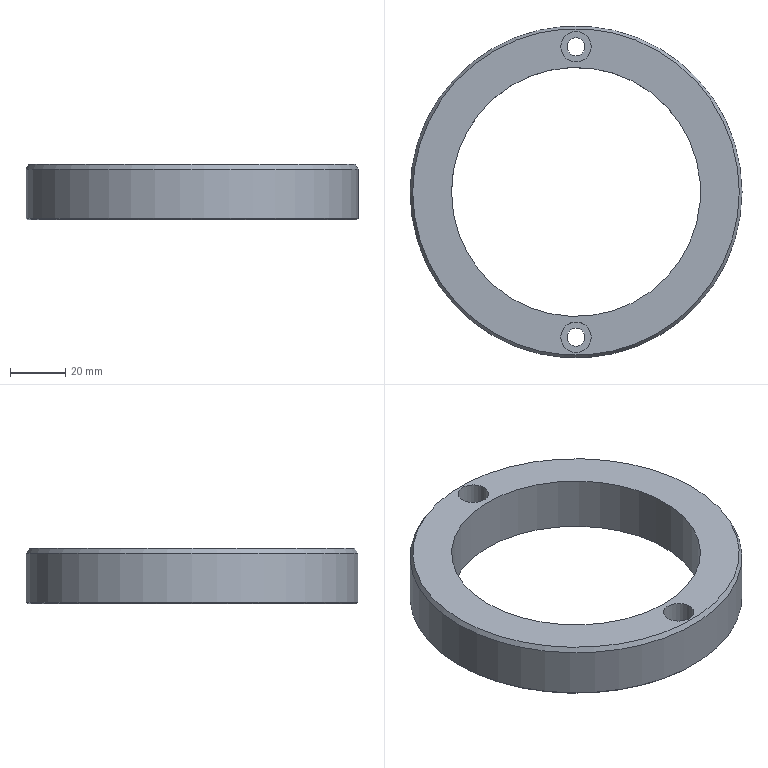Part | STEP file | 1_id506_xmt_txt | 1 solid | 12 faces | box 120 x 120 x 20 mm | volume 95777 mm3 | cylinder 6 | plane 4 | cone 2 | commonest cylinder face diameters 6.5 x2 11 x2 90 x1 120 x1
STEP:
#1=CARTESIAN_POINT('',(60.,90.,199.268));
#2=VERTEX_POINT('',#1);
#3=CARTESIAN_POINT('',(0.,90.,199.268));
#4=DIRECTION('',(0.,0.,1.));
#5=DIRECTION('',(1.,0.,0.));
#6=AXIS2_PLACEMENT_3D('',#3,#4,#5);
#7=CIRCLE('',#6,60.);
#8=EDGE_CURVE('',#2,#2,#7,.T.);
#9=ORIENTED_EDGE('',*,*,#8,.T.);
#10=EDGE_LOOP('',(#9));
#11=FACE_BOUND('',#10,.T.);
#12=CARTESIAN_POINT('',(59.,90.,201.));
#13=VERTEX_POINT('',#12);
#14=CARTESIAN_POINT('',(0.,90.,201.));
#15=DIRECTION('',(0.,0.,-1.));
#16=DIRECTION('',(1.,0.,0.));
#17=AXIS2_PLACEMENT_3D('',#14,#15,#16);
#18=CIRCLE('',#17,59.);
#19=EDGE_CURVE('',#13,#13,#18,.T.);
#20=ORIENTED_EDGE('',*,*,#19,.T.);
#21=EDGE_LOOP('',(#20));
#22=FACE_BOUND('',#21,.T.);
#23=CARTESIAN_POINT('',(0.,90.,201.));
#24=DIRECTION('',(0.,0.,-1.));
#25=DIRECTION('',(-1.,0.,0.));
#26=AXIS2_PLACEMENT_3D('',#23,#24,#25);
#27=CONICAL_SURFACE('',#26,59.,30.);
#28=ADVANCED_FACE('',(#11,#22),#27,.T.);
#29=ORIENTED_EDGE('',*,*,#8,.F.);
#30=EDGE_LOOP('',(#29));
#31=FACE_BOUND('',#30,.T.);
#32=CARTESIAN_POINT('',(60.,90.,181.5));
#33=VERTEX_POINT('',#32);
#34=CARTESIAN_POINT('',(0.,90.,181.5));
#35=DIRECTION('',(0.,0.,-1.));
#36=DIRECTION('',(1.,0.,0.));
#37=AXIS2_PLACEMENT_3D('',#34,#35,#36);
#38=CIRCLE('',#37,60.);
#39=EDGE_CURVE('',#33,#33,#38,.T.);
#40=ORIENTED_EDGE('',*,*,#39,.F.);
#41=EDGE_LOOP('',(#40));
#42=FACE_BOUND('',#41,.T.);
#43=CARTESIAN_POINT('',(0.,90.,191.));
#44=DIRECTION('',(0.,0.,-1.));
#45=DIRECTION('',(1.,0.,0.));
#46=AXIS2_PLACEMENT_3D('',#43,#44,#45);
#47=CYLINDRICAL_SURFACE('',#46,60.);
#48=ADVANCED_FACE('',(#31,#42),#47,.T.);
#49=ORIENTED_EDGE('',*,*,#39,.T.);
#50=EDGE_LOOP('',(#49));
#51=FACE_BOUND('',#50,.T.);
#52=CARTESIAN_POINT('',(59.5,90.,181.));
#53=VERTEX_POINT('',#52);
#54=CARTESIAN_POINT('',(0.,90.,181.));
#55=DIRECTION('',(0.,0.,1.));
#56=DIRECTION('',(1.,0.,0.));
#57=AXIS2_PLACEMENT_3D('',#54,#55,#56);
#58=CIRCLE('',#57,59.5);
#59=EDGE_CURVE('',#53,#53,#58,.T.);
#60=ORIENTED_EDGE('',*,*,#59,.T.);
#61=EDGE_LOOP('',(#60));
#62=FACE_BOUND('',#61,.T.);
#63=CARTESIAN_POINT('',(0.,90.,181.));
#64=DIRECTION('',(0.,0.,1.));
#65=DIRECTION('',(-1.,0.,0.));
#66=AXIS2_PLACEMENT_3D('',#63,#64,#65);
#67=CONICAL_SURFACE('',#66,59.5,45.);
#68=ADVANCED_FACE('',(#51,#62),#67,.T.);
#69=CARTESIAN_POINT('',(5.5,37.5,189.));
#70=VERTEX_POINT('',#69);
#71=CARTESIAN_POINT('',(0.,37.5,189.));
#72=DIRECTION('',(0.,0.,-1.));
#73=DIRECTION('',(1.,0.,0.));
#74=AXIS2_PLACEMENT_3D('',#71,#72,#73);
#75=CIRCLE('',#74,5.5);
#76=EDGE_CURVE('',#70,#70,#75,.T.);
#77=ORIENTED_EDGE('',*,*,#76,.T.);
#78=EDGE_LOOP('',(#77));
#79=FACE_BOUND('',#78,.T.);
#80=CARTESIAN_POINT('',(5.5,37.5,201.));
#81=VERTEX_POINT('',#80);
#82=CARTESIAN_POINT('',(0.,37.5,201.));
#83=DIRECTION('',(0.,0.,-1.));
#84=DIRECTION('',(1.,0.,0.));
#85=AXIS2_PLACEMENT_3D('',#82,#83,#84);
#86=CIRCLE('',#85,5.5);
#87=EDGE_CURVE('',#81,#81,#86,.T.);
#88=ORIENTED_EDGE('',*,*,#87,.F.);
#89=EDGE_LOOP('',(#88));
#90=FACE_BOUND('',#89,.T.);
#91=CARTESIAN_POINT('',(0.,37.5,195.));
#92=DIRECTION('',(0.,0.,-1.));
#93=DIRECTION('',(-1.,0.,0.));
#94=AXIS2_PLACEMENT_3D('',#91,#92,#93);
#95=CYLINDRICAL_SURFACE('',#94,5.5);
#96=ADVANCED_FACE('',(#79,#90),#95,.F.);
#97=CARTESIAN_POINT('',(3.25,37.5,181.));
#98=VERTEX_POINT('',#97);
#99=CARTESIAN_POINT('',(0.,37.5,181.));
#100=DIRECTION('',(0.,0.,1.));
#101=DIRECTION('',(1.,0.,0.));
#102=AXIS2_PLACEMENT_3D('',#99,#100,#101);
#103=CIRCLE('',#102,3.25);
#104=EDGE_CURVE('',#98,#98,#103,.T.);
#105=ORIENTED_EDGE('',*,*,#104,.F.);
#106=EDGE_LOOP('',(#105));
#107=FACE_BOUND('',#106,.T.);
#108=CARTESIAN_POINT('',(3.25,37.5,189.));
#109=VERTEX_POINT('',#108);
#110=CARTESIAN_POINT('',(0.,37.5,189.));
#111=DIRECTION('',(0.,0.,1.));
#112=DIRECTION('',(1.,0.,0.));
#113=AXIS2_PLACEMENT_3D('',#110,#111,#112);
#114=CIRCLE('',#113,3.25);
#115=EDGE_CURVE('',#109,#109,#114,.T.);
#116=ORIENTED_EDGE('',*,*,#115,.T.);
#117=EDGE_LOOP('',(#116));
#118=FACE_BOUND('',#117,.T.);
#119=CARTESIAN_POINT('',(0.,37.5,191.));
#120=DIRECTION('',(0.,0.,-1.));
#121=DIRECTION('',(-1.,0.,0.));
#122=AXIS2_PLACEMENT_3D('',#119,#120,#121);
#123=CYLINDRICAL_SURFACE('',#122,3.25);
#124=ADVANCED_FACE('',(#107,#118),#123,.F.);
#125=CARTESIAN_POINT('',(-5.5,142.5,189.));
#126=VERTEX_POINT('',#125);
#127=CARTESIAN_POINT('',(0.,142.5,189.));
#128=DIRECTION('',(0.,0.,-1.));
#129=DIRECTION('',(-1.,0.,0.));
#130=AXIS2_PLACEMENT_3D('',#127,#128,#129);
#131=CIRCLE('',#130,5.5);
#132=EDGE_CURVE('',#126,#126,#131,.T.);
#133=ORIENTED_EDGE('',*,*,#132,.T.);
#134=EDGE_LOOP('',(#133));
#135=FACE_BOUND('',#134,.T.);
#136=CARTESIAN_POINT('',(-5.5,142.5,201.));
#137=VERTEX_POINT('',#136);
#138=CARTESIAN_POINT('',(0.,142.5,201.));
#139=DIRECTION('',(0.,0.,-1.));
#140=DIRECTION('',(-1.,0.,0.));
#141=AXIS2_PLACEMENT_3D('',#138,#139,#140);
#142=CIRCLE('',#141,5.5);
#143=EDGE_CURVE('',#137,#137,#142,.T.);
#144=ORIENTED_EDGE('',*,*,#143,.F.);
#145=EDGE_LOOP('',(#144));
#146=FACE_BOUND('',#145,.T.);
#147=CARTESIAN_POINT('',(0.,142.5,195.));
#148=DIRECTION('',(0.,0.,-1.));
#149=DIRECTION('',(1.,0.,0.));
#150=AXIS2_PLACEMENT_3D('',#147,#148,#149);
#151=CYLINDRICAL_SURFACE('',#150,5.5);
#152=ADVANCED_FACE('',(#135,#146),#151,.F.);
#153=CARTESIAN_POINT('',(-3.25,142.5,181.));
#154=VERTEX_POINT('',#153);
#155=CARTESIAN_POINT('',(0.,142.5,181.));
#156=DIRECTION('',(0.,0.,1.));
#157=DIRECTION('',(-1.,0.,0.));
#158=AXIS2_PLACEMENT_3D('',#155,#156,#157);
#159=CIRCLE('',#158,3.25);
#160=EDGE_CURVE('',#154,#154,#159,.T.);
#161=ORIENTED_EDGE('',*,*,#160,.F.);
#162=EDGE_LOOP('',(#161));
#163=FACE_BOUND('',#162,.T.);
#164=CARTESIAN_POINT('',(-3.25,142.5,189.));
#165=VERTEX_POINT('',#164);
#166=CARTESIAN_POINT('',(0.,142.5,189.));
#167=DIRECTION('',(0.,0.,1.));
#168=DIRECTION('',(-1.,0.,0.));
#169=AXIS2_PLACEMENT_3D('',#166,#167,#168);
#170=CIRCLE('',#169,3.25);
#171=EDGE_CURVE('',#165,#165,#170,.T.);
#172=ORIENTED_EDGE('',*,*,#171,.T.);
#173=EDGE_LOOP('',(#172));
#174=FACE_BOUND('',#173,.T.);
#175=CARTESIAN_POINT('',(0.,142.5,191.));
#176=DIRECTION('',(0.,0.,-1.));
#177=DIRECTION('',(1.,0.,0.));
#178=AXIS2_PLACEMENT_3D('',#175,#176,#177);
#179=CYLINDRICAL_SURFACE('',#178,3.25);
#180=ADVANCED_FACE('',(#163,#174),#179,.F.);
#181=CARTESIAN_POINT('',(-45.,90.,181.));
#182=VERTEX_POINT('',#181);
#183=CARTESIAN_POINT('',(0.,90.,181.));
#184=DIRECTION('',(0.,0.,1.));
#185=DIRECTION('',(-1.,0.,0.));
#186=AXIS2_PLACEMENT_3D('',#183,#184,#185);
#187=CIRCLE('',#186,45.);
#188=EDGE_CURVE('',#182,#182,#187,.T.);
#189=ORIENTED_EDGE('',*,*,#188,.F.);
#190=EDGE_LOOP('',(#189));
#191=FACE_BOUND('',#190,.T.);
#192=CARTESIAN_POINT('',(-45.,90.,201.));
#193=VERTEX_POINT('',#192);
#194=CARTESIAN_POINT('',(0.,90.,201.));
#195=DIRECTION('',(0.,0.,-1.));
#196=DIRECTION('',(-1.,0.,0.));
#197=AXIS2_PLACEMENT_3D('',#194,#195,#196);
#198=CIRCLE('',#197,45.);
#199=EDGE_CURVE('',#193,#193,#198,.T.);
#200=ORIENTED_EDGE('',*,*,#199,.F.);
#201=EDGE_LOOP('',(#200));
#202=FACE_BOUND('',#201,.T.);
#203=CARTESIAN_POINT('',(0.,90.,191.));
#204=DIRECTION('',(0.,0.,-1.));
#205=DIRECTION('',(1.,0.,0.));
#206=AXIS2_PLACEMENT_3D('',#203,#204,#205);
#207=CYLINDRICAL_SURFACE('',#206,45.);
#208=ADVANCED_FACE('',(#191,#202),#207,.F.);
#209=ORIENTED_EDGE('',*,*,#171,.F.);
#210=EDGE_LOOP('',(#209));
#211=FACE_BOUND('',#210,.T.);
#212=ORIENTED_EDGE('',*,*,#132,.F.);
#213=EDGE_LOOP('',(#212));
#214=FACE_BOUND('',#213,.T.);
#215=CARTESIAN_POINT('',(0.,142.5,189.));
#216=DIRECTION('',(0.,0.,-1.));
#217=DIRECTION('',(1.,0.,0.));
#218=AXIS2_PLACEMENT_3D('',#215,#216,#217);
#219=PLANE('',#218);
#220=ADVANCED_FACE('',(#211,#214),#219,.F.);
#221=ORIENTED_EDGE('',*,*,#115,.F.);
#222=EDGE_LOOP('',(#221));
#223=FACE_BOUND('',#222,.T.);
#224=ORIENTED_EDGE('',*,*,#76,.F.);
#225=EDGE_LOOP('',(#224));
#226=FACE_BOUND('',#225,.T.);
#227=CARTESIAN_POINT('',(0.,37.5,189.));
#228=DIRECTION('',(0.,0.,-1.));
#229=DIRECTION('',(-1.,0.,0.));
#230=AXIS2_PLACEMENT_3D('',#227,#228,#229);
#231=PLANE('',#230);
#232=ADVANCED_FACE('',(#223,#226),#231,.F.);
#233=ORIENTED_EDGE('',*,*,#188,.T.);
#234=EDGE_LOOP('',(#233));
#235=FACE_BOUND('',#234,.T.);
#236=ORIENTED_EDGE('',*,*,#59,.F.);
#237=EDGE_LOOP('',(#236));
#238=FACE_BOUND('',#237,.T.);
#239=ORIENTED_EDGE('',*,*,#104,.T.);
#240=EDGE_LOOP('',(#239));
#241=FACE_BOUND('',#240,.T.);
#242=ORIENTED_EDGE('',*,*,#160,.T.);
#243=EDGE_LOOP('',(#242));
#244=FACE_BOUND('',#243,.T.);
#245=CARTESIAN_POINT('',(0.,90.,181.));
#246=DIRECTION('',(0.,0.,-1.));
#247=DIRECTION('',(1.,0.,0.));
#248=AXIS2_PLACEMENT_3D('',#245,#246,#247);
#249=PLANE('',#248);
#250=ADVANCED_FACE('',(#235,#238,#241,#244),#249,.T.);
#251=ORIENTED_EDGE('',*,*,#199,.T.);
#252=EDGE_LOOP('',(#251));
#253=FACE_BOUND('',#252,.T.);
#254=ORIENTED_EDGE('',*,*,#19,.F.);
#255=EDGE_LOOP('',(#254));
#256=FACE_BOUND('',#255,.T.);
#257=ORIENTED_EDGE('',*,*,#87,.T.);
#258=EDGE_LOOP('',(#257));
#259=FACE_BOUND('',#258,.T.);
#260=ORIENTED_EDGE('',*,*,#143,.T.);
#261=EDGE_LOOP('',(#260));
#262=FACE_BOUND('',#261,.T.);
#263=CARTESIAN_POINT('',(0.,90.,201.));
#264=DIRECTION('',(0.,0.,1.));
#265=DIRECTION('',(-1.,0.,0.));
#266=AXIS2_PLACEMENT_3D('',#263,#264,#265);
#267=PLANE('',#266);
#268=ADVANCED_FACE('',(#253,#256,#259,#262),#267,.T.);
#269=CLOSED_SHELL('',(#28,#48,#68,#96,#124,#152,#180,#208,#220,#232,#250,#268));
#270=MANIFOLD_SOLID_BREP('',#269);
#271=(LENGTH_UNIT()NAMED_UNIT(*)SI_UNIT(.MILLI.,.METRE.));
#272=UNCERTAINTY_MEASURE_WITH_UNIT(LENGTH_MEASURE(0.00002),#271,'','');
#273=(NAMED_UNIT(*)PLANE_ANGLE_UNIT()SI_UNIT($,.RADIAN.));
#274=PLANE_ANGLE_MEASURE_WITH_UNIT(PLANE_ANGLE_MEASURE(0.01745),#273);
#275=DIMENSIONAL_EXPONENTS(0.,0.,0.,0.,0.,0.,0.);
#276=(CONVERSION_BASED_UNIT('DEGREE',#274)NAMED_UNIT(#275)PLANE_ANGLE_UNIT());
#277=(NAMED_UNIT(*)SI_UNIT($,.STERADIAN.)SOLID_ANGLE_UNIT());
#278=(GEOMETRIC_REPRESENTATION_CONTEXT(3)GLOBAL_UNCERTAINTY_ASSIGNED_CONTEXT((#272))GLOBAL_UNIT_ASSIGNED_CONTEXT((#271,#276,#277))REPRESENTATION_CONTEXT('',''));
#279=ADVANCED_BREP_SHAPE_REPRESENTATION('',(#270),#278);